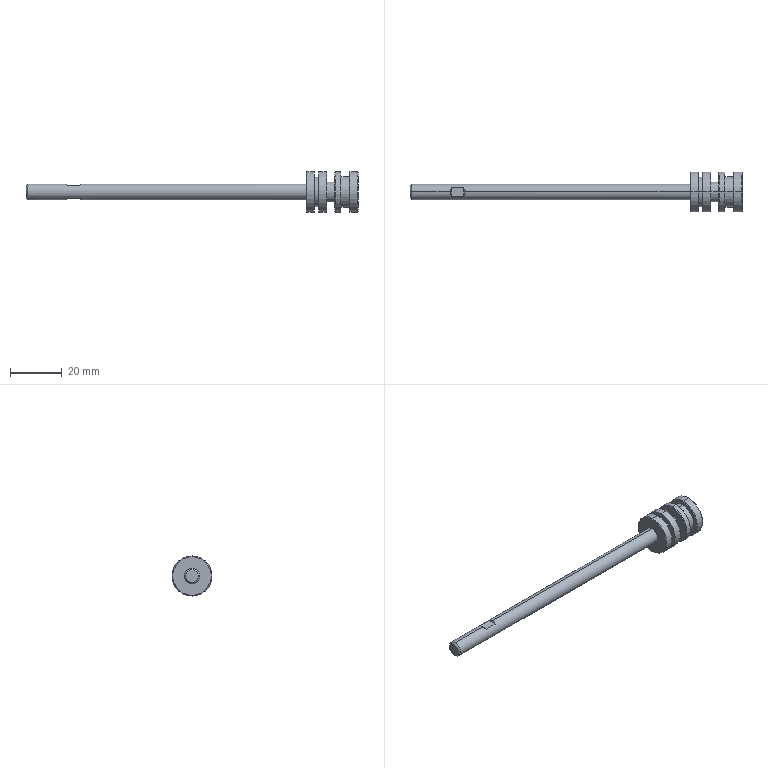Part | STEP file | 16LBMA50_Rod | 1 solid | 45 faces | box 128 x 15.5 x 15.5 mm | volume 5968 mm3 | cylinder 16 | plane 15 | cone 14 | commonest cylinder face diameters 15.5 x8 6 x2 7.7 x2 11.4 x2 11.9 x2